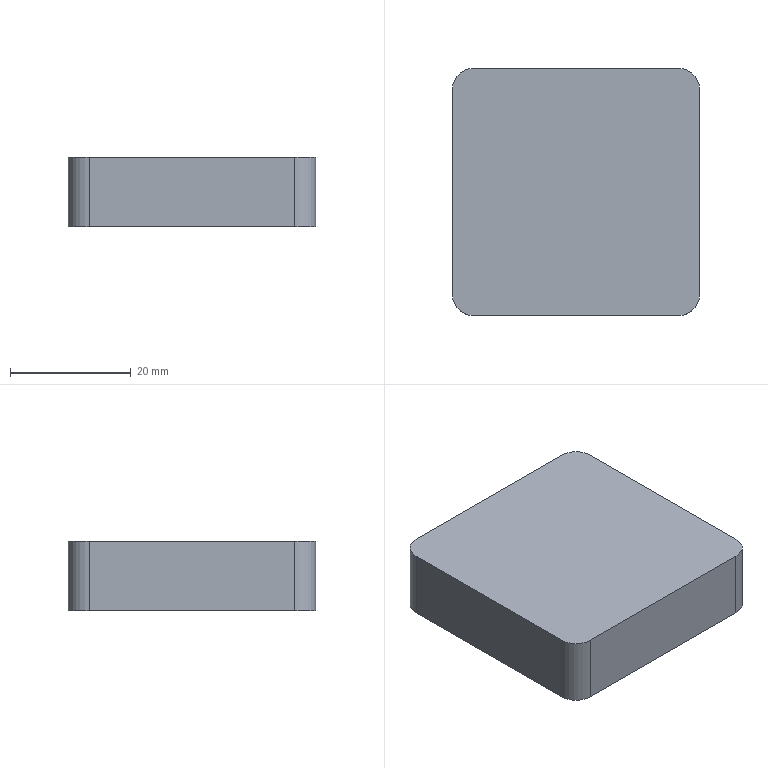Part | SolidWorks | features BaseBody 1 | 1 solid | 10 faces | box 41 x 41 x 11.5 mm | volume 19211 mm3 | plane 6 | cylinder 4 | commonest cylinder face diameters 7 x4
STEP:
#1=CARTESIAN_POINT('',(11.921,-15.625,11.5));
#2=VERTEX_POINT('',#1);
#3=CARTESIAN_POINT('',(11.921,18.375,11.5));
#4=VERTEX_POINT('',#3);
#5=CARTESIAN_POINT('',(11.921,1.375,11.5));
#6=DIRECTION('',(0.,1.,0.));
#7=VECTOR('',#6,1000.);
#8=LINE('',#5,#7);
#9=EDGE_CURVE('',#2,#4,#8,.T.);
#10=ORIENTED_EDGE('',*,*,#9,.T.);
#11=CARTESIAN_POINT('',(8.421,21.875,11.5));
#12=VERTEX_POINT('',#11);
#13=CARTESIAN_POINT('',(8.421,18.375,11.5));
#14=DIRECTION('',(0.,0.,1.));
#15=DIRECTION('',(1.,0.,0.));
#16=AXIS2_PLACEMENT_3D('',#13,#14,#15);
#17=CIRCLE('',#16,3.5);
#18=EDGE_CURVE('',#4,#12,#17,.T.);
#19=ORIENTED_EDGE('',*,*,#18,.T.);
#20=CARTESIAN_POINT('',(-25.579,21.875,11.5));
#21=VERTEX_POINT('',#20);
#22=CARTESIAN_POINT('',(-8.579,21.875,11.5));
#23=DIRECTION('',(-1.,0.,0.));
#24=VECTOR('',#23,1000.);
#25=LINE('',#22,#24);
#26=EDGE_CURVE('',#12,#21,#25,.T.);
#27=ORIENTED_EDGE('',*,*,#26,.T.);
#28=CARTESIAN_POINT('',(-29.079,18.375,11.5));
#29=VERTEX_POINT('',#28);
#30=CARTESIAN_POINT('',(-25.579,18.375,11.5));
#31=DIRECTION('',(0.,0.,1.));
#32=DIRECTION('',(1.,0.,0.));
#33=AXIS2_PLACEMENT_3D('',#30,#31,#32);
#34=CIRCLE('',#33,3.5);
#35=EDGE_CURVE('',#21,#29,#34,.T.);
#36=ORIENTED_EDGE('',*,*,#35,.T.);
#37=CARTESIAN_POINT('',(-29.079,-15.625,11.5));
#38=VERTEX_POINT('',#37);
#39=CARTESIAN_POINT('',(-29.079,1.375,11.5));
#40=DIRECTION('',(0.,-1.,0.));
#41=VECTOR('',#40,1000.);
#42=LINE('',#39,#41);
#43=EDGE_CURVE('',#29,#38,#42,.T.);
#44=ORIENTED_EDGE('',*,*,#43,.T.);
#45=CARTESIAN_POINT('',(-25.579,-19.125,11.5));
#46=VERTEX_POINT('',#45);
#47=CARTESIAN_POINT('',(-25.579,-15.625,11.5));
#48=DIRECTION('',(0.,0.,1.));
#49=DIRECTION('',(1.,0.,0.));
#50=AXIS2_PLACEMENT_3D('',#47,#48,#49);
#51=CIRCLE('',#50,3.5);
#52=EDGE_CURVE('',#38,#46,#51,.T.);
#53=ORIENTED_EDGE('',*,*,#52,.T.);
#54=CARTESIAN_POINT('',(8.421,-19.125,11.5));
#55=VERTEX_POINT('',#54);
#56=CARTESIAN_POINT('',(-8.579,-19.125,11.5));
#57=DIRECTION('',(1.,0.,0.));
#58=VECTOR('',#57,1000.);
#59=LINE('',#56,#58);
#60=EDGE_CURVE('',#46,#55,#59,.T.);
#61=ORIENTED_EDGE('',*,*,#60,.T.);
#62=CARTESIAN_POINT('',(8.421,-15.625,11.5));
#63=DIRECTION('',(0.,0.,1.));
#64=DIRECTION('',(1.,0.,0.));
#65=AXIS2_PLACEMENT_3D('',#62,#63,#64);
#66=CIRCLE('',#65,3.5);
#67=EDGE_CURVE('',#55,#2,#66,.T.);
#68=ORIENTED_EDGE('',*,*,#67,.T.);
#69=EDGE_LOOP('',(#10,#19,#27,#36,#44,#53,#61,#68));
#70=FACE_OUTER_BOUND('',#69,.T.);
#71=CARTESIAN_POINT('',(-8.579,1.375,11.5));
#72=DIRECTION('',(0.,0.,1.));
#73=DIRECTION('',(1.,0.,0.));
#74=AXIS2_PLACEMENT_3D('',#71,#72,#73);
#75=PLANE('',#74);
#76=ADVANCED_FACE('',(#70),#75,.T.);
#77=CARTESIAN_POINT('',(11.921,18.375,0.));
#78=VERTEX_POINT('',#77);
#79=CARTESIAN_POINT('',(8.421,21.875,0.));
#80=VERTEX_POINT('',#79);
#81=CARTESIAN_POINT('',(8.421,18.375,0.));
#82=DIRECTION('',(0.,0.,1.));
#83=DIRECTION('',(1.,0.,0.));
#84=AXIS2_PLACEMENT_3D('',#81,#82,#83);
#85=CIRCLE('',#84,3.5);
#86=EDGE_CURVE('',#78,#80,#85,.T.);
#87=ORIENTED_EDGE('',*,*,#86,.T.);
#88=CARTESIAN_POINT('',(8.421,21.875,0.));
#89=DIRECTION('',(0.,0.,1.));
#90=VECTOR('',#89,1000.);
#91=LINE('',#88,#90);
#92=EDGE_CURVE('',#80,#12,#91,.T.);
#93=ORIENTED_EDGE('',*,*,#92,.T.);
#94=ORIENTED_EDGE('',*,*,#18,.F.);
#95=CARTESIAN_POINT('',(11.921,18.375,0.));
#96=DIRECTION('',(0.,0.,-1.));
#97=VECTOR('',#96,1000.);
#98=LINE('',#95,#97);
#99=EDGE_CURVE('',#4,#78,#98,.T.);
#100=ORIENTED_EDGE('',*,*,#99,.T.);
#101=EDGE_LOOP('',(#87,#93,#94,#100));
#102=FACE_OUTER_BOUND('',#101,.T.);
#103=CARTESIAN_POINT('',(8.421,18.375,0.));
#104=DIRECTION('',(0.,0.,1.));
#105=DIRECTION('',(1.,0.,0.));
#106=AXIS2_PLACEMENT_3D('',#103,#104,#105);
#107=CYLINDRICAL_SURFACE('',#106,3.5);
#108=ADVANCED_FACE('',(#102),#107,.T.);
#109=CARTESIAN_POINT('',(11.921,-15.625,0.));
#110=VERTEX_POINT('',#109);
#111=CARTESIAN_POINT('',(11.921,18.375,0.));
#112=DIRECTION('',(0.,1.,0.));
#113=VECTOR('',#112,1000.);
#114=LINE('',#111,#113);
#115=EDGE_CURVE('',#110,#78,#114,.T.);
#116=ORIENTED_EDGE('',*,*,#115,.T.);
#117=ORIENTED_EDGE('',*,*,#99,.F.);
#118=ORIENTED_EDGE('',*,*,#9,.F.);
#119=CARTESIAN_POINT('',(11.921,-15.625,0.));
#120=DIRECTION('',(0.,0.,-1.));
#121=VECTOR('',#120,1000.);
#122=LINE('',#119,#121);
#123=EDGE_CURVE('',#2,#110,#122,.T.);
#124=ORIENTED_EDGE('',*,*,#123,.T.);
#125=EDGE_LOOP('',(#116,#117,#118,#124));
#126=FACE_OUTER_BOUND('',#125,.T.);
#127=CARTESIAN_POINT('',(11.921,18.375,0.));
#128=DIRECTION('',(1.,0.,0.));
#129=DIRECTION('',(0.,0.,-1.));
#130=AXIS2_PLACEMENT_3D('',#127,#128,#129);
#131=PLANE('',#130);
#132=ADVANCED_FACE('',(#126),#131,.T.);
#133=CARTESIAN_POINT('',(8.421,-19.125,0.));
#134=VERTEX_POINT('',#133);
#135=CARTESIAN_POINT('',(8.421,-15.625,0.));
#136=DIRECTION('',(0.,0.,1.));
#137=DIRECTION('',(1.,0.,0.));
#138=AXIS2_PLACEMENT_3D('',#135,#136,#137);
#139=CIRCLE('',#138,3.5);
#140=EDGE_CURVE('',#134,#110,#139,.T.);
#141=ORIENTED_EDGE('',*,*,#140,.T.);
#142=ORIENTED_EDGE('',*,*,#123,.F.);
#143=ORIENTED_EDGE('',*,*,#67,.F.);
#144=CARTESIAN_POINT('',(8.421,-19.125,0.));
#145=DIRECTION('',(0.,0.,-1.));
#146=VECTOR('',#145,1000.);
#147=LINE('',#144,#146);
#148=EDGE_CURVE('',#55,#134,#147,.T.);
#149=ORIENTED_EDGE('',*,*,#148,.T.);
#150=EDGE_LOOP('',(#141,#142,#143,#149));
#151=FACE_OUTER_BOUND('',#150,.T.);
#152=CARTESIAN_POINT('',(8.421,-15.625,0.));
#153=DIRECTION('',(0.,0.,1.));
#154=DIRECTION('',(1.,0.,0.));
#155=AXIS2_PLACEMENT_3D('',#152,#153,#154);
#156=CYLINDRICAL_SURFACE('',#155,3.5);
#157=ADVANCED_FACE('',(#151),#156,.T.);
#158=CARTESIAN_POINT('',(-25.579,-19.125,0.));
#159=VERTEX_POINT('',#158);
#160=CARTESIAN_POINT('',(8.421,-19.125,0.));
#161=DIRECTION('',(1.,0.,0.));
#162=VECTOR('',#161,1000.);
#163=LINE('',#160,#162);
#164=EDGE_CURVE('',#159,#134,#163,.T.);
#165=ORIENTED_EDGE('',*,*,#164,.T.);
#166=ORIENTED_EDGE('',*,*,#148,.F.);
#167=ORIENTED_EDGE('',*,*,#60,.F.);
#168=CARTESIAN_POINT('',(-25.579,-19.125,0.));
#169=DIRECTION('',(0.,0.,-1.));
#170=VECTOR('',#169,1000.);
#171=LINE('',#168,#170);
#172=EDGE_CURVE('',#46,#159,#171,.T.);
#173=ORIENTED_EDGE('',*,*,#172,.T.);
#174=EDGE_LOOP('',(#165,#166,#167,#173));
#175=FACE_OUTER_BOUND('',#174,.T.);
#176=CARTESIAN_POINT('',(8.421,-19.125,0.));
#177=DIRECTION('',(0.,-1.,0.));
#178=DIRECTION('',(0.,0.,-1.));
#179=AXIS2_PLACEMENT_3D('',#176,#177,#178);
#180=PLANE('',#179);
#181=ADVANCED_FACE('',(#175),#180,.T.);
#182=CARTESIAN_POINT('',(-29.079,-15.625,0.));
#183=VERTEX_POINT('',#182);
#184=CARTESIAN_POINT('',(-25.579,-15.625,0.));
#185=DIRECTION('',(0.,0.,1.));
#186=DIRECTION('',(1.,0.,0.));
#187=AXIS2_PLACEMENT_3D('',#184,#185,#186);
#188=CIRCLE('',#187,3.5);
#189=EDGE_CURVE('',#183,#159,#188,.T.);
#190=ORIENTED_EDGE('',*,*,#189,.T.);
#191=ORIENTED_EDGE('',*,*,#172,.F.);
#192=ORIENTED_EDGE('',*,*,#52,.F.);
#193=CARTESIAN_POINT('',(-29.079,-15.625,0.));
#194=DIRECTION('',(0.,0.,-1.));
#195=VECTOR('',#194,1000.);
#196=LINE('',#193,#195);
#197=EDGE_CURVE('',#38,#183,#196,.T.);
#198=ORIENTED_EDGE('',*,*,#197,.T.);
#199=EDGE_LOOP('',(#190,#191,#192,#198));
#200=FACE_OUTER_BOUND('',#199,.T.);
#201=CARTESIAN_POINT('',(-25.579,-15.625,0.));
#202=DIRECTION('',(0.,0.,1.));
#203=DIRECTION('',(1.,0.,0.));
#204=AXIS2_PLACEMENT_3D('',#201,#202,#203);
#205=CYLINDRICAL_SURFACE('',#204,3.5);
#206=ADVANCED_FACE('',(#200),#205,.T.);
#207=CARTESIAN_POINT('',(-29.079,18.375,0.));
#208=VERTEX_POINT('',#207);
#209=CARTESIAN_POINT('',(-29.079,-15.625,0.));
#210=DIRECTION('',(0.,-1.,0.));
#211=VECTOR('',#210,1000.);
#212=LINE('',#209,#211);
#213=EDGE_CURVE('',#208,#183,#212,.T.);
#214=ORIENTED_EDGE('',*,*,#213,.T.);
#215=ORIENTED_EDGE('',*,*,#197,.F.);
#216=ORIENTED_EDGE('',*,*,#43,.F.);
#217=CARTESIAN_POINT('',(-29.079,18.375,0.));
#218=DIRECTION('',(0.,0.,-1.));
#219=VECTOR('',#218,1000.);
#220=LINE('',#217,#219);
#221=EDGE_CURVE('',#29,#208,#220,.T.);
#222=ORIENTED_EDGE('',*,*,#221,.T.);
#223=EDGE_LOOP('',(#214,#215,#216,#222));
#224=FACE_OUTER_BOUND('',#223,.T.);
#225=CARTESIAN_POINT('',(-29.079,-15.625,0.));
#226=DIRECTION('',(-1.,0.,0.));
#227=DIRECTION('',(0.,0.,1.));
#228=AXIS2_PLACEMENT_3D('',#225,#226,#227);
#229=PLANE('',#228);
#230=ADVANCED_FACE('',(#224),#229,.T.);
#231=CARTESIAN_POINT('',(-25.579,21.875,0.));
#232=VERTEX_POINT('',#231);
#233=CARTESIAN_POINT('',(-25.579,18.375,0.));
#234=DIRECTION('',(0.,0.,1.));
#235=DIRECTION('',(1.,0.,0.));
#236=AXIS2_PLACEMENT_3D('',#233,#234,#235);
#237=CIRCLE('',#236,3.5);
#238=EDGE_CURVE('',#232,#208,#237,.T.);
#239=ORIENTED_EDGE('',*,*,#238,.T.);
#240=ORIENTED_EDGE('',*,*,#221,.F.);
#241=ORIENTED_EDGE('',*,*,#35,.F.);
#242=CARTESIAN_POINT('',(-25.579,21.875,0.));
#243=DIRECTION('',(0.,0.,-1.));
#244=VECTOR('',#243,1000.);
#245=LINE('',#242,#244);
#246=EDGE_CURVE('',#21,#232,#245,.T.);
#247=ORIENTED_EDGE('',*,*,#246,.T.);
#248=EDGE_LOOP('',(#239,#240,#241,#247));
#249=FACE_OUTER_BOUND('',#248,.T.);
#250=CARTESIAN_POINT('',(-25.579,18.375,0.));
#251=DIRECTION('',(0.,0.,1.));
#252=DIRECTION('',(1.,0.,0.));
#253=AXIS2_PLACEMENT_3D('',#250,#251,#252);
#254=CYLINDRICAL_SURFACE('',#253,3.5);
#255=ADVANCED_FACE('',(#249),#254,.T.);
#256=CARTESIAN_POINT('',(-25.579,21.875,0.));
#257=DIRECTION('',(-1.,0.,0.));
#258=VECTOR('',#257,1000.);
#259=LINE('',#256,#258);
#260=EDGE_CURVE('',#80,#232,#259,.T.);
#261=ORIENTED_EDGE('',*,*,#260,.T.);
#262=ORIENTED_EDGE('',*,*,#246,.F.);
#263=ORIENTED_EDGE('',*,*,#26,.F.);
#264=ORIENTED_EDGE('',*,*,#92,.F.);
#265=EDGE_LOOP('',(#261,#262,#263,#264));
#266=FACE_OUTER_BOUND('',#265,.T.);
#267=CARTESIAN_POINT('',(-25.579,21.875,0.));
#268=DIRECTION('',(0.,1.,0.));
#269=DIRECTION('',(0.,0.,1.));
#270=AXIS2_PLACEMENT_3D('',#267,#268,#269);
#271=PLANE('',#270);
#272=ADVANCED_FACE('',(#266),#271,.T.);
#273=ORIENTED_EDGE('',*,*,#260,.F.);
#274=ORIENTED_EDGE('',*,*,#86,.F.);
#275=ORIENTED_EDGE('',*,*,#115,.F.);
#276=ORIENTED_EDGE('',*,*,#140,.F.);
#277=ORIENTED_EDGE('',*,*,#164,.F.);
#278=ORIENTED_EDGE('',*,*,#189,.F.);
#279=ORIENTED_EDGE('',*,*,#213,.F.);
#280=ORIENTED_EDGE('',*,*,#238,.F.);
#281=EDGE_LOOP('',(#273,#274,#275,#276,#277,#278,#279,#280));
#282=FACE_OUTER_BOUND('',#281,.T.);
#283=CARTESIAN_POINT('',(-8.579,1.375,0.));
#284=DIRECTION('',(0.,0.,1.));
#285=DIRECTION('',(1.,0.,0.));
#286=AXIS2_PLACEMENT_3D('',#283,#284,#285);
#287=PLANE('',#286);
#288=ADVANCED_FACE('',(#282),#287,.F.);
#289=CLOSED_SHELL('',(#76,#108,#132,#157,#181,#206,#230,#255,#272,#288));
#290=MANIFOLD_SOLID_BREP('',#289);
#291=CARTESIAN_POINT('',(0.,0.,0.));
#292=DIRECTION('',(0.,0.,1.));
#293=DIRECTION('',(1.,0.,0.));
#294=AXIS2_PLACEMENT_3D('',#291,#292,#293);
#295=(LENGTH_UNIT()NAMED_UNIT(*)SI_UNIT(.MILLI.,.METRE.));
#296=UNCERTAINTY_MEASURE_WITH_UNIT(LENGTH_MEASURE(0.00001),#295,'','');
#297=(NAMED_UNIT(*)PLANE_ANGLE_UNIT()SI_UNIT($,.RADIAN.));
#298=(NAMED_UNIT(*)SI_UNIT($,.STERADIAN.)SOLID_ANGLE_UNIT());
#299=(GEOMETRIC_REPRESENTATION_CONTEXT(3)GLOBAL_UNCERTAINTY_ASSIGNED_CONTEXT((#296))GLOBAL_UNIT_ASSIGNED_CONTEXT((#295,#297,#298))REPRESENTATION_CONTEXT('',''));
#300=ADVANCED_BREP_SHAPE_REPRESENTATION('',(#290,#294),#299);